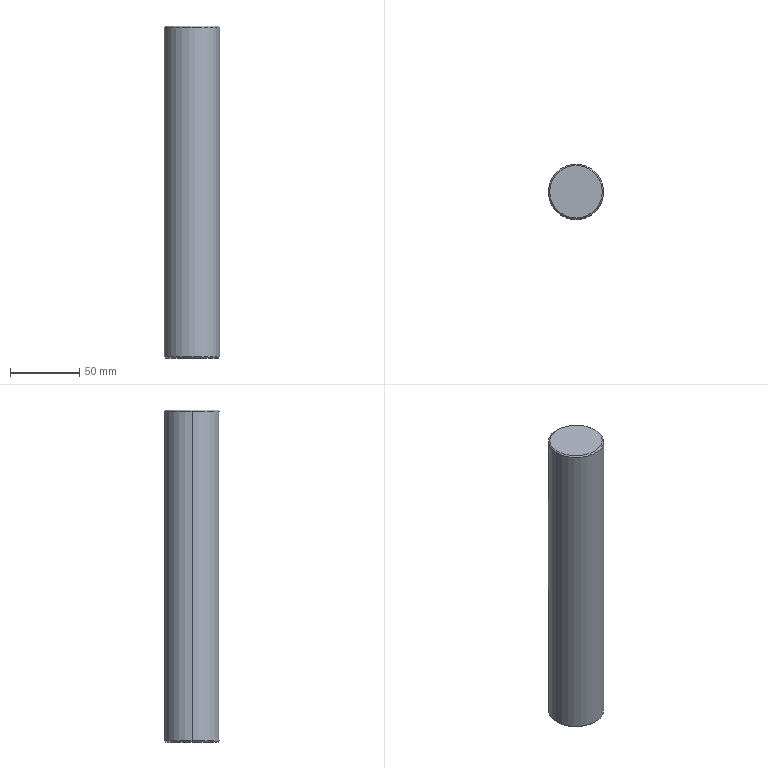Part | NX | features BREP 1 | 1 solid | 8 faces | box 40 x 40 x 240 mm | volume 301469 mm3 | cone 4 | cylinder 2 | plane 2 | commonest cylinder face diameters 40 x2
STEP:
#1=CARTESIAN_POINT('',(-19.,0.,0.));
#2=VERTEX_POINT('',#1);
#3=CARTESIAN_POINT('',(19.,0.,0.));
#4=VERTEX_POINT('',#3);
#5=CARTESIAN_POINT('',(0.,0.,0.));
#6=DIRECTION('',(0.,0.,-1.));
#7=DIRECTION('',(1.,0.,0.));
#8=AXIS2_PLACEMENT_3D('',#5,#6,#7);
#9=CIRCLE('',#8,19.);
#10=EDGE_CURVE('',#2,#4,#9,.T.);
#11=ORIENTED_EDGE('',*,*,#10,.F.);
#12=CARTESIAN_POINT('',(-20.,0.,1.));
#13=VERTEX_POINT('',#12);
#14=CARTESIAN_POINT('',(-20.,0.,1.));
#15=DIRECTION('',(-0.7071,0.,0.7071));
#16=VECTOR('',#15,1000.);
#17=LINE('',#14,#16);
#18=EDGE_CURVE('',#13,#2,#17,.F.);
#19=ORIENTED_EDGE('',*,*,#18,.F.);
#20=CARTESIAN_POINT('',(20.,0.,1.));
#21=VERTEX_POINT('',#20);
#22=CARTESIAN_POINT('',(0.,0.,1.));
#23=DIRECTION('',(0.,0.,1.));
#24=DIRECTION('',(1.,0.,0.));
#25=AXIS2_PLACEMENT_3D('',#22,#23,#24);
#26=CIRCLE('',#25,20.);
#27=EDGE_CURVE('',#21,#13,#26,.T.);
#28=ORIENTED_EDGE('',*,*,#27,.F.);
#29=CARTESIAN_POINT('',(20.,0.,1.));
#30=DIRECTION('',(0.7071,0.,0.7071));
#31=VECTOR('',#30,1000.);
#32=LINE('',#29,#31);
#33=EDGE_CURVE('',#21,#4,#32,.F.);
#34=ORIENTED_EDGE('',*,*,#33,.T.);
#35=EDGE_LOOP('',(#11,#19,#28,#34));
#36=FACE_BOUND('',#35,.T.);
#37=CARTESIAN_POINT('',(0.,0.,1.));
#38=DIRECTION('',(0.,0.,1.));
#39=DIRECTION('',(1.,0.,0.));
#40=AXIS2_PLACEMENT_3D('',#37,#38,#39);
#41=CONICAL_SURFACE('',#40,20.,0.7854);
#42=ADVANCED_FACE('',(#36),#41,.T.);
#43=CARTESIAN_POINT('',(19.,0.,240.));
#44=VERTEX_POINT('',#43);
#45=CARTESIAN_POINT('',(-19.,0.,240.));
#46=VERTEX_POINT('',#45);
#47=CARTESIAN_POINT('',(0.,0.,240.));
#48=DIRECTION('',(0.,0.,1.));
#49=DIRECTION('',(1.,0.,0.));
#50=AXIS2_PLACEMENT_3D('',#47,#48,#49);
#51=CIRCLE('',#50,19.);
#52=EDGE_CURVE('',#44,#46,#51,.T.);
#53=ORIENTED_EDGE('',*,*,#52,.F.);
#54=CARTESIAN_POINT('',(20.,0.,239.));
#55=VERTEX_POINT('',#54);
#56=CARTESIAN_POINT('',(19.,0.,240.));
#57=DIRECTION('',(0.7071,0.,-0.7071));
#58=VECTOR('',#57,1000.);
#59=LINE('',#56,#58);
#60=EDGE_CURVE('',#44,#55,#59,.T.);
#61=ORIENTED_EDGE('',*,*,#60,.T.);
#62=CARTESIAN_POINT('',(-20.,0.,239.));
#63=VERTEX_POINT('',#62);
#64=CARTESIAN_POINT('',(0.,0.,239.));
#65=DIRECTION('',(0.,0.,-1.));
#66=DIRECTION('',(1.,0.,0.));
#67=AXIS2_PLACEMENT_3D('',#64,#65,#66);
#68=CIRCLE('',#67,20.);
#69=EDGE_CURVE('',#63,#55,#68,.T.);
#70=ORIENTED_EDGE('',*,*,#69,.F.);
#71=CARTESIAN_POINT('',(-19.,0.,240.));
#72=DIRECTION('',(-0.7071,0.,-0.7071));
#73=VECTOR('',#72,1000.);
#74=LINE('',#71,#73);
#75=EDGE_CURVE('',#46,#63,#74,.T.);
#76=ORIENTED_EDGE('',*,*,#75,.F.);
#77=EDGE_LOOP('',(#53,#61,#70,#76));
#78=FACE_BOUND('',#77,.T.);
#79=CARTESIAN_POINT('',(0.,0.,240.));
#80=DIRECTION('',(0.,0.,-1.));
#81=DIRECTION('',(-1.,0.,0.));
#82=AXIS2_PLACEMENT_3D('',#79,#80,#81);
#83=CONICAL_SURFACE('',#82,19.,0.7854);
#84=ADVANCED_FACE('',(#78),#83,.T.);
#85=ORIENTED_EDGE('',*,*,#69,.T.);
#86=CARTESIAN_POINT('',(20.,0.,240.));
#87=DIRECTION('',(0.,0.,-1.));
#88=VECTOR('',#87,1000.);
#89=LINE('',#86,#88);
#90=EDGE_CURVE('',#55,#21,#89,.T.);
#91=ORIENTED_EDGE('',*,*,#90,.T.);
#92=ORIENTED_EDGE('',*,*,#27,.T.);
#93=CARTESIAN_POINT('',(-20.,0.,240.));
#94=DIRECTION('',(0.,0.,-1.));
#95=VECTOR('',#94,1000.);
#96=LINE('',#93,#95);
#97=EDGE_CURVE('',#63,#13,#96,.T.);
#98=ORIENTED_EDGE('',*,*,#97,.F.);
#99=EDGE_LOOP('',(#85,#91,#92,#98));
#100=FACE_BOUND('',#99,.T.);
#101=CARTESIAN_POINT('',(0.,0.,240.));
#102=DIRECTION('',(0.,0.,-1.));
#103=DIRECTION('',(-1.,0.,0.));
#104=AXIS2_PLACEMENT_3D('',#101,#102,#103);
#105=CYLINDRICAL_SURFACE('',#104,20.);
#106=ADVANCED_FACE('',(#100),#105,.T.);
#107=ORIENTED_EDGE('',*,*,#90,.F.);
#108=CARTESIAN_POINT('',(0.,0.,239.));
#109=DIRECTION('',(0.,0.,-1.));
#110=DIRECTION('',(1.,0.,0.));
#111=AXIS2_PLACEMENT_3D('',#108,#109,#110);
#112=CIRCLE('',#111,20.);
#113=EDGE_CURVE('',#55,#63,#112,.T.);
#114=ORIENTED_EDGE('',*,*,#113,.T.);
#115=ORIENTED_EDGE('',*,*,#97,.T.);
#116=CARTESIAN_POINT('',(0.,0.,1.));
#117=DIRECTION('',(0.,0.,1.));
#118=DIRECTION('',(1.,0.,0.));
#119=AXIS2_PLACEMENT_3D('',#116,#117,#118);
#120=CIRCLE('',#119,20.);
#121=EDGE_CURVE('',#13,#21,#120,.T.);
#122=ORIENTED_EDGE('',*,*,#121,.T.);
#123=EDGE_LOOP('',(#107,#114,#115,#122));
#124=FACE_BOUND('',#123,.T.);
#125=CARTESIAN_POINT('',(0.,0.,240.));
#126=DIRECTION('',(0.,0.,-1.));
#127=DIRECTION('',(-1.,0.,0.));
#128=AXIS2_PLACEMENT_3D('',#125,#126,#127);
#129=CYLINDRICAL_SURFACE('',#128,20.);
#130=ADVANCED_FACE('',(#124),#129,.T.);
#131=CARTESIAN_POINT('',(0.,0.,240.));
#132=DIRECTION('',(0.,0.,1.));
#133=DIRECTION('',(1.,0.,0.));
#134=AXIS2_PLACEMENT_3D('',#131,#132,#133);
#135=CIRCLE('',#134,19.);
#136=EDGE_CURVE('',#46,#44,#135,.T.);
#137=ORIENTED_EDGE('',*,*,#136,.T.);
#138=ORIENTED_EDGE('',*,*,#52,.T.);
#139=EDGE_LOOP('',(#137,#138));
#140=FACE_BOUND('',#139,.T.);
#141=CARTESIAN_POINT('',(0.,0.,240.));
#142=DIRECTION('',(0.,0.,1.));
#143=DIRECTION('',(1.,0.,0.));
#144=AXIS2_PLACEMENT_3D('',#141,#142,#143);
#145=PLANE('',#144);
#146=ADVANCED_FACE('',(#140),#145,.T.);
#147=CARTESIAN_POINT('',(0.,0.,0.));
#148=DIRECTION('',(0.,0.,-1.));
#149=DIRECTION('',(1.,0.,0.));
#150=AXIS2_PLACEMENT_3D('',#147,#148,#149);
#151=CIRCLE('',#150,19.);
#152=EDGE_CURVE('',#4,#2,#151,.T.);
#153=ORIENTED_EDGE('',*,*,#152,.T.);
#154=ORIENTED_EDGE('',*,*,#10,.T.);
#155=EDGE_LOOP('',(#153,#154));
#156=FACE_BOUND('',#155,.T.);
#157=CARTESIAN_POINT('',(0.,0.,0.));
#158=DIRECTION('',(0.,0.,1.));
#159=DIRECTION('',(1.,0.,0.));
#160=AXIS2_PLACEMENT_3D('',#157,#158,#159);
#161=PLANE('',#160);
#162=ADVANCED_FACE('',(#156),#161,.F.);
#163=ORIENTED_EDGE('',*,*,#60,.F.);
#164=ORIENTED_EDGE('',*,*,#136,.F.);
#165=ORIENTED_EDGE('',*,*,#75,.T.);
#166=ORIENTED_EDGE('',*,*,#113,.F.);
#167=EDGE_LOOP('',(#163,#164,#165,#166));
#168=FACE_BOUND('',#167,.T.);
#169=CARTESIAN_POINT('',(0.,0.,240.));
#170=DIRECTION('',(0.,0.,-1.));
#171=DIRECTION('',(-1.,0.,0.));
#172=AXIS2_PLACEMENT_3D('',#169,#170,#171);
#173=CONICAL_SURFACE('',#172,19.,0.7854);
#174=ADVANCED_FACE('',(#168),#173,.T.);
#175=ORIENTED_EDGE('',*,*,#18,.T.);
#176=ORIENTED_EDGE('',*,*,#152,.F.);
#177=ORIENTED_EDGE('',*,*,#33,.F.);
#178=ORIENTED_EDGE('',*,*,#121,.F.);
#179=EDGE_LOOP('',(#175,#176,#177,#178));
#180=FACE_BOUND('',#179,.T.);
#181=CARTESIAN_POINT('',(0.,0.,1.));
#182=DIRECTION('',(0.,0.,1.));
#183=DIRECTION('',(1.,0.,0.));
#184=AXIS2_PLACEMENT_3D('',#181,#182,#183);
#185=CONICAL_SURFACE('',#184,20.,0.7854);
#186=ADVANCED_FACE('',(#180),#185,.T.);
#187=CLOSED_SHELL('',(#42,#84,#106,#130,#146,#162,#174,#186));
#188=MANIFOLD_SOLID_BREP('',#187);
#189=(LENGTH_UNIT()NAMED_UNIT(*)SI_UNIT(.MILLI.,.METRE.));
#190=UNCERTAINTY_MEASURE_WITH_UNIT(LENGTH_MEASURE(0.00001),#189,'','');
#191=(NAMED_UNIT(*)PLANE_ANGLE_UNIT()SI_UNIT($,.RADIAN.));
#192=(NAMED_UNIT(*)SI_UNIT($,.STERADIAN.)SOLID_ANGLE_UNIT());
#193=(GEOMETRIC_REPRESENTATION_CONTEXT(3)GLOBAL_UNCERTAINTY_ASSIGNED_CONTEXT((#190))GLOBAL_UNIT_ASSIGNED_CONTEXT((#189,#191,#192))REPRESENTATION_CONTEXT('',''));
#194=ADVANCED_BREP_SHAPE_REPRESENTATION('',(#188),#193);